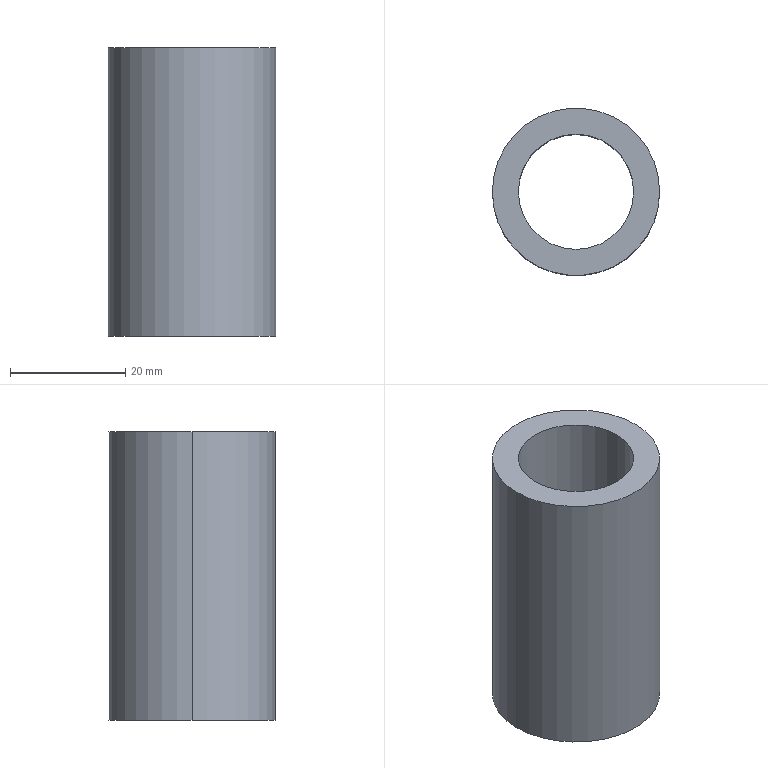Part | SolidWorks | features Extrusion 1 | 1 solid | 6 faces | box 29 x 29 x 50 mm | volume 17318 mm3 | cylinder 4 | plane 2 | commonest cylinder face diameters 20 x2 29 x2
STEP:
#1=CARTESIAN_POINT('',(-10.,0.,50.));
#2=VERTEX_POINT('',#1);
#3=CARTESIAN_POINT('',(10.,0.,50.));
#4=VERTEX_POINT('',#3);
#5=CARTESIAN_POINT('',(0.,0.,50.));
#6=DIRECTION('',(0.,0.,1.));
#7=DIRECTION('',(1.,0.,0.));
#8=AXIS2_PLACEMENT_3D('',#5,#6,#7);
#9=CIRCLE('',#8,10.);
#10=EDGE_CURVE('',#2,#4,#9,.T.);
#11=ORIENTED_EDGE('',*,*,#10,.T.);
#12=CARTESIAN_POINT('',(10.,0.,0.));
#13=VERTEX_POINT('',#12);
#14=CARTESIAN_POINT('',(10.,0.,50.));
#15=DIRECTION('',(0.,0.,-1.));
#16=VECTOR('',#15,1000.);
#17=LINE('',#14,#16);
#18=EDGE_CURVE('',#4,#13,#17,.T.);
#19=ORIENTED_EDGE('',*,*,#18,.T.);
#20=CARTESIAN_POINT('',(-10.,0.,0.));
#21=VERTEX_POINT('',#20);
#22=CARTESIAN_POINT('',(0.,0.,0.));
#23=DIRECTION('',(0.,0.,1.));
#24=DIRECTION('',(1.,0.,0.));
#25=AXIS2_PLACEMENT_3D('',#22,#23,#24);
#26=CIRCLE('',#25,10.);
#27=EDGE_CURVE('',#21,#13,#26,.T.);
#28=ORIENTED_EDGE('',*,*,#27,.F.);
#29=CARTESIAN_POINT('',(-10.,0.,50.));
#30=DIRECTION('',(0.,0.,-1.));
#31=VECTOR('',#30,1000.);
#32=LINE('',#29,#31);
#33=EDGE_CURVE('',#2,#21,#32,.T.);
#34=ORIENTED_EDGE('',*,*,#33,.F.);
#35=EDGE_LOOP('',(#11,#19,#28,#34));
#36=FACE_OUTER_BOUND('',#35,.T.);
#37=CARTESIAN_POINT('',(0.,0.,50.));
#38=DIRECTION('',(0.,0.,-1.));
#39=DIRECTION('',(-1.,0.,0.));
#40=AXIS2_PLACEMENT_3D('',#37,#38,#39);
#41=CYLINDRICAL_SURFACE('',#40,10.);
#42=ADVANCED_FACE('',(#36),#41,.F.);
#43=CARTESIAN_POINT('',(14.5,0.,50.));
#44=VERTEX_POINT('',#43);
#45=CARTESIAN_POINT('',(-14.5,0.,50.));
#46=VERTEX_POINT('',#45);
#47=CARTESIAN_POINT('',(0.,0.,50.));
#48=DIRECTION('',(0.,0.,1.));
#49=DIRECTION('',(1.,0.,0.));
#50=AXIS2_PLACEMENT_3D('',#47,#48,#49);
#51=CIRCLE('',#50,14.5);
#52=EDGE_CURVE('',#44,#46,#51,.T.);
#53=ORIENTED_EDGE('',*,*,#52,.F.);
#54=CARTESIAN_POINT('',(14.5,0.,0.));
#55=VERTEX_POINT('',#54);
#56=CARTESIAN_POINT('',(14.5,0.,50.));
#57=DIRECTION('',(0.,0.,-1.));
#58=VECTOR('',#57,1000.);
#59=LINE('',#56,#58);
#60=EDGE_CURVE('',#44,#55,#59,.T.);
#61=ORIENTED_EDGE('',*,*,#60,.T.);
#62=CARTESIAN_POINT('',(-14.5,0.,0.));
#63=VERTEX_POINT('',#62);
#64=CARTESIAN_POINT('',(0.,0.,0.));
#65=DIRECTION('',(0.,0.,1.));
#66=DIRECTION('',(1.,0.,0.));
#67=AXIS2_PLACEMENT_3D('',#64,#65,#66);
#68=CIRCLE('',#67,14.5);
#69=EDGE_CURVE('',#55,#63,#68,.T.);
#70=ORIENTED_EDGE('',*,*,#69,.T.);
#71=CARTESIAN_POINT('',(-14.5,0.,50.));
#72=DIRECTION('',(0.,0.,-1.));
#73=VECTOR('',#72,1000.);
#74=LINE('',#71,#73);
#75=EDGE_CURVE('',#46,#63,#74,.T.);
#76=ORIENTED_EDGE('',*,*,#75,.F.);
#77=EDGE_LOOP('',(#53,#61,#70,#76));
#78=FACE_OUTER_BOUND('',#77,.T.);
#79=CARTESIAN_POINT('',(0.,0.,50.));
#80=DIRECTION('',(0.,0.,-1.));
#81=DIRECTION('',(-1.,0.,0.));
#82=AXIS2_PLACEMENT_3D('',#79,#80,#81);
#83=CYLINDRICAL_SURFACE('',#82,14.5);
#84=ADVANCED_FACE('',(#78),#83,.T.);
#85=CARTESIAN_POINT('',(0.,0.,50.));
#86=DIRECTION('',(0.,0.,1.));
#87=DIRECTION('',(1.,0.,0.));
#88=AXIS2_PLACEMENT_3D('',#85,#86,#87);
#89=CIRCLE('',#88,14.5);
#90=EDGE_CURVE('',#46,#44,#89,.T.);
#91=ORIENTED_EDGE('',*,*,#90,.T.);
#92=ORIENTED_EDGE('',*,*,#52,.T.);
#93=EDGE_LOOP('',(#91,#92));
#94=FACE_OUTER_BOUND('',#93,.T.);
#95=ORIENTED_EDGE('',*,*,#10,.F.);
#96=CARTESIAN_POINT('',(0.,0.,50.));
#97=DIRECTION('',(0.,0.,1.));
#98=DIRECTION('',(1.,0.,0.));
#99=AXIS2_PLACEMENT_3D('',#96,#97,#98);
#100=CIRCLE('',#99,10.);
#101=EDGE_CURVE('',#4,#2,#100,.T.);
#102=ORIENTED_EDGE('',*,*,#101,.F.);
#103=EDGE_LOOP('',(#95,#102));
#104=FACE_BOUND('',#103,.T.);
#105=CARTESIAN_POINT('',(0.,0.,50.));
#106=DIRECTION('',(0.,0.,1.));
#107=DIRECTION('',(1.,0.,0.));
#108=AXIS2_PLACEMENT_3D('',#105,#106,#107);
#109=PLANE('',#108);
#110=ADVANCED_FACE('',(#94,#104),#109,.T.);
#111=CARTESIAN_POINT('',(0.,0.,0.));
#112=DIRECTION('',(0.,0.,1.));
#113=DIRECTION('',(1.,0.,0.));
#114=AXIS2_PLACEMENT_3D('',#111,#112,#113);
#115=CIRCLE('',#114,14.5);
#116=EDGE_CURVE('',#63,#55,#115,.T.);
#117=ORIENTED_EDGE('',*,*,#116,.F.);
#118=ORIENTED_EDGE('',*,*,#69,.F.);
#119=EDGE_LOOP('',(#117,#118));
#120=FACE_OUTER_BOUND('',#119,.T.);
#121=ORIENTED_EDGE('',*,*,#27,.T.);
#122=CARTESIAN_POINT('',(0.,0.,0.));
#123=DIRECTION('',(0.,0.,1.));
#124=DIRECTION('',(1.,0.,0.));
#125=AXIS2_PLACEMENT_3D('',#122,#123,#124);
#126=CIRCLE('',#125,10.);
#127=EDGE_CURVE('',#13,#21,#126,.T.);
#128=ORIENTED_EDGE('',*,*,#127,.T.);
#129=EDGE_LOOP('',(#121,#128));
#130=FACE_BOUND('',#129,.T.);
#131=CARTESIAN_POINT('',(0.,0.,0.));
#132=DIRECTION('',(0.,0.,1.));
#133=DIRECTION('',(1.,0.,0.));
#134=AXIS2_PLACEMENT_3D('',#131,#132,#133);
#135=PLANE('',#134);
#136=ADVANCED_FACE('',(#120,#130),#135,.F.);
#137=ORIENTED_EDGE('',*,*,#60,.F.);
#138=ORIENTED_EDGE('',*,*,#90,.F.);
#139=ORIENTED_EDGE('',*,*,#75,.T.);
#140=ORIENTED_EDGE('',*,*,#116,.T.);
#141=EDGE_LOOP('',(#137,#138,#139,#140));
#142=FACE_OUTER_BOUND('',#141,.T.);
#143=CARTESIAN_POINT('',(0.,0.,50.));
#144=DIRECTION('',(0.,0.,-1.));
#145=DIRECTION('',(-1.,0.,0.));
#146=AXIS2_PLACEMENT_3D('',#143,#144,#145);
#147=CYLINDRICAL_SURFACE('',#146,14.5);
#148=ADVANCED_FACE('',(#142),#147,.T.);
#149=ORIENTED_EDGE('',*,*,#18,.F.);
#150=ORIENTED_EDGE('',*,*,#101,.T.);
#151=ORIENTED_EDGE('',*,*,#33,.T.);
#152=ORIENTED_EDGE('',*,*,#127,.F.);
#153=EDGE_LOOP('',(#149,#150,#151,#152));
#154=FACE_OUTER_BOUND('',#153,.T.);
#155=CARTESIAN_POINT('',(0.,0.,50.));
#156=DIRECTION('',(0.,0.,-1.));
#157=DIRECTION('',(-1.,0.,0.));
#158=AXIS2_PLACEMENT_3D('',#155,#156,#157);
#159=CYLINDRICAL_SURFACE('',#158,10.);
#160=ADVANCED_FACE('',(#154),#159,.F.);
#161=CLOSED_SHELL('',(#42,#84,#110,#136,#148,#160));
#162=MANIFOLD_SOLID_BREP('',#161);
#163=CARTESIAN_POINT('',(0.,0.,0.));
#164=DIRECTION('',(0.,0.,1.));
#165=DIRECTION('',(1.,0.,0.));
#166=AXIS2_PLACEMENT_3D('',#163,#164,#165);
#167=(LENGTH_UNIT()NAMED_UNIT(*)SI_UNIT(.MILLI.,.METRE.));
#168=UNCERTAINTY_MEASURE_WITH_UNIT(LENGTH_MEASURE(0.00001),#167,'','');
#169=(NAMED_UNIT(*)PLANE_ANGLE_UNIT()SI_UNIT($,.RADIAN.));
#170=(NAMED_UNIT(*)SI_UNIT($,.STERADIAN.)SOLID_ANGLE_UNIT());
#171=(GEOMETRIC_REPRESENTATION_CONTEXT(3)GLOBAL_UNCERTAINTY_ASSIGNED_CONTEXT((#168))GLOBAL_UNIT_ASSIGNED_CONTEXT((#167,#169,#170))REPRESENTATION_CONTEXT('',''));
#172=ADVANCED_BREP_SHAPE_REPRESENTATION('',(#162,#166),#171);